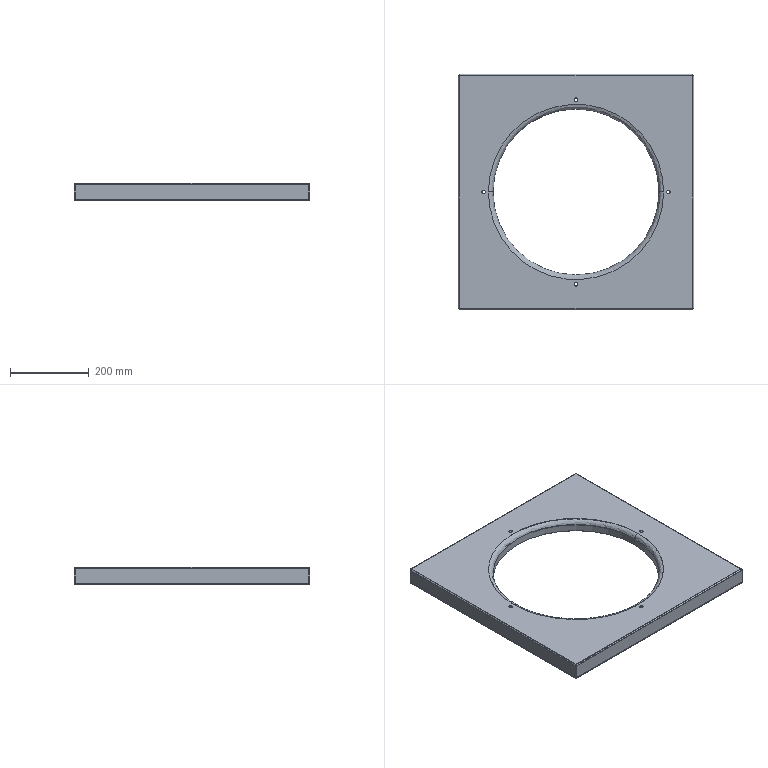Part | STEP file | 750038408 | 1 solid | 71 faces | box 600 x 600 x 44 mm | volume 824704 mm3 | plane 39 | cylinder 28 | spline 4 | commonest cylinder face diameters 4 x8 8 x8 9 x8 422 x2 426 x2